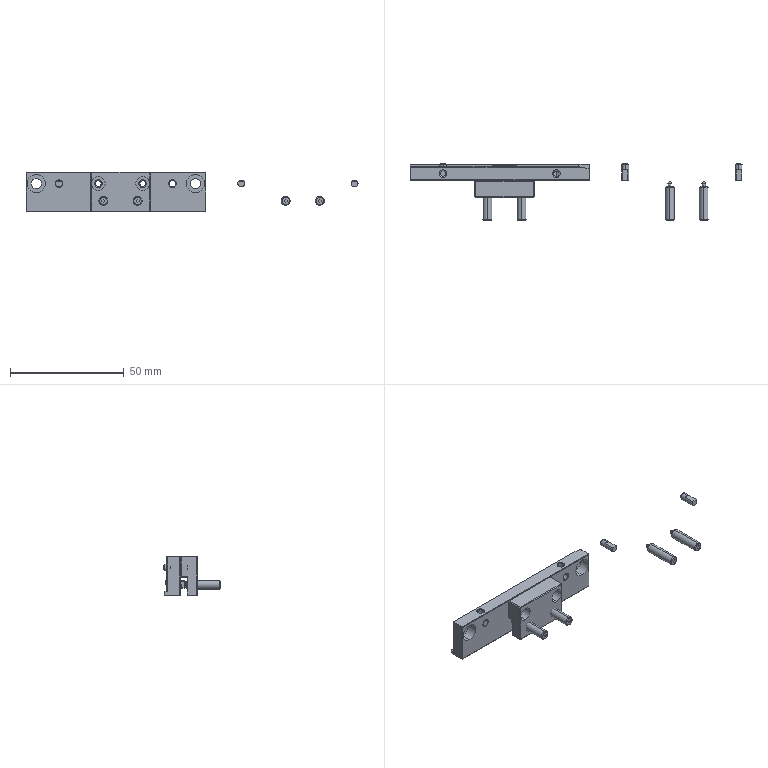Part | NX | 12 solids | 262 faces | box 145.781 x 25.105 x 17.4 mm | volume 11449 mm3 | plane 140 | cylinder 74 | cone 42 | sphere 6 | commonest cylinder face diameters 1.6 x12 3.2 x12 4 x12 3 x10 2.5 x8 3.3 x4